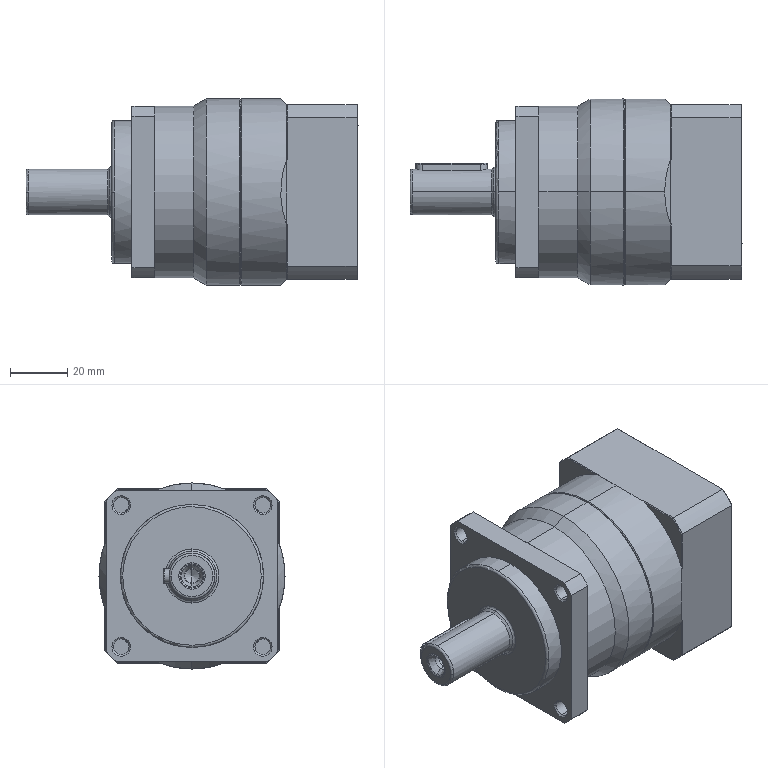Part | SolidWorks | features BaseBody 3 | 3 solids | 259 faces | box 116 x 65 x 65 mm | volume 248255 mm3 | plane 85 | cylinder 85 | cone 70 | torus 19 | commonest cylinder face diameters 4.2 x8 4.5 x8 5.5 x8 7.5 x8 80 x8 50 x7